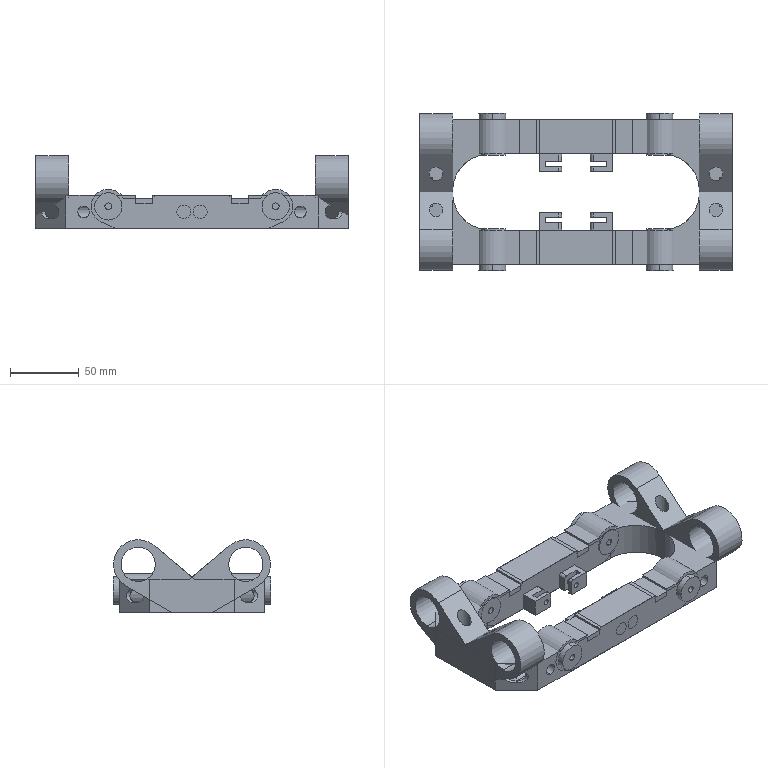NC program | Mastercam | posted with a generic post | part box 228 x 114.503 x 53 mm
Lines 1 to 1812 of 27132, first 1622 of 1812 lines:
%
:0001()
(MATERIAL - ALUMINUM MM - 2024)
(T24|100 FEM |H24)
(T16|16 FEM |H16|XY STOCK TO LEAVE - .15|Z STOCK TO LEAVE - 0.)
(T7|6 CHM |H7)
(T11|10 DR |H11)
(T23|50 FEM |H23|XY STOCK TO LEAVE - .3|Z STOCK TO LEAVE - 0.)
(T10|10 FEM |H10|XY STOCK TO LEAVE - .01|Z STOCK TO LEAVE - 0.)
(T9|10 DR |H9)
(T12|12 FEM |H12|XY STOCK TO LEAVE - .5|Z STOCK TO LEAVE - .2)
(T5|5 DR |H5)
(T6|6 FEM |H6|XY STOCK TO LEAVE - -.05|Z STOCK TO LEAVE - 0.)
(T13|10 BNOS |H13)
(T17|5 BM/BNOS |H17)
N100 G21
N102 G0 G17 G40 G80 G90 G94 G98
N104 G0 G28 G91 Z0.
N106 G0 G28 X0. Y0.
(100 FEM |TOOL - 24|DIA. OFF. - 24|LEN. - 24|TOOL DIA. - 100.)
N108 T24 M6
N110 G0 G54 G90 X-184. Y34.998 C0. B0. S4000 M3
N112 G43 H24 Z25.
N114 Z10.
N116 G1 Z0. F600.
N118 X134. F1200.
N120 G2 X168.998 Y0. J-34.998
N122 X134. Y-34.998 I-34.998
N124 G1 X-184.
N126 G0 Z25.
N128 M5
N130 G0 G28 G91 Z0.
N132 G28
N134 M01
N136 G0 G17 G40 G80 G90 G94 G98
N138 G0 G28 G91 Z0.
(16 FEM |TOOL - 16|DIA. OFF. - 16|LEN. - 16|TOOL DIA. - 16.)
N140 T16 M6
N142 G0 G54 G90 X-123.705 Y-71.319 C0. B0. S8250 M3
N144 G43 H16 Z50.
N146 Z3.
N148 G1 Z-53.3 F600.
N150 X-124.522 Y-69.286 F4000.
N152 X-125.029 Y-68.026
N154 G3 X-125.824 Y-66.824 I-3.34 J-1.343
N156 G1 X-126.147 Y-66.363
N158 X-126.473 Y-65.871
N160 X-126.833 Y-65.268
N162 X-127.184 Y-64.581
N164 X-127.476 Y-63.894
N166 X-127.702 Y-63.25
N168 X-127.876 Y-62.65
N170 X-128.009 Y-62.093
N172 X-128.112 Y-61.577
N174 X-128.191 Y-61.096
N176 X-128.298 Y-60.248
N178 X-128.365 Y-59.48
N180 X-128.407 Y-58.772
N182 G2 X-128.45 Y-57.477 I47.576 J2.234
N184 X-128.471 Y-55.217 I122.465 J2.26
N186 G1 Y-55.116
N188 G2 X-128.462 Y-51.17 I996.713 J-.393
N190 G1 X-128.46 Y-50.609
N192 X-128.25 Y5.613
N194 X-128.058 Y56.95
N196 X-128.05 Y57.685
N198 X-128.029 Y58.177
N200 X-127.985 Y58.725
N202 X-127.91 Y59.316
N204 X-127.797 Y59.933
N206 X-127.642 Y60.566
N208 X-127.44 Y61.204
N210 X-127.19 Y61.835
N212 X-126.891 Y62.451
N214 X-126.547 Y63.041
N216 X-126.165 Y63.599
N218 X-125.751 Y64.122
N220 X-125.311 Y64.608
N222 X-124.851 Y65.056
N224 X-124.376 Y65.466
N226 X-123.892 Y65.839
N228 X-123.404 Y66.177
N230 X-122.914 Y66.482
N232 X-122.426 Y66.755
N234 X-121.942 Y67.
N236 X-121.464 Y67.219
N238 X-120.994 Y67.415
N240 X-120.532 Y67.589
N242 X-120.08 Y67.744
N244 X-119.637 Y67.881
N246 X-119.204 Y68.004
N248 X-118.382 Y68.207
N250 X-117.593 Y68.369
N252 X-116.834 Y68.498
N254 X-116.102 Y68.602
N256 X-115.395 Y68.685
N258 X-114.709 Y68.752
N260 G2 X-113.389 Y68.851 I4.24 J-48.055
N262 X-111.506 Y68.939 I4.246 J-70.131
N264 X-108.513 Y69.008 I4.662 J-138.634
N266 X-103.882 Y69.041 I5.546 J-453.218
N268 G1 X-103.309 Y69.042
N270 X-98.736 Y69.048
N272 X-55.423 Y69.05
N274 X1.563
N276 X58.549
N278 X115.535
N280 X116.118
N282 X116.955 Y69.034
N284 X117.484 Y69.001
N286 X118.06 Y68.941
N288 X118.668 Y68.845
N290 X119.297 Y68.708
N292 X119.935 Y68.526
N294 X120.57 Y68.296
N296 X121.194 Y68.018
N298 X121.796 Y67.693
N300 X122.368 Y67.326
N302 X122.906 Y66.925
N304 X123.408 Y66.495
N306 X123.872 Y66.042
N308 X124.298 Y65.573
N310 X124.687 Y65.092
N312 X125.039 Y64.605
N314 X125.357 Y64.115
N316 X125.644 Y63.626
N318 X125.901 Y63.14
N320 X126.13 Y62.66
N322 X126.335 Y62.187
N324 X126.518 Y61.721
N326 X126.681 Y61.265
N328 X126.825 Y60.818
N330 X126.954 Y60.381
N332 X127.069 Y59.953
N334 X127.259 Y59.141
N336 X127.41 Y58.361
N338 X127.531 Y57.61
N340 X127.629 Y56.886
N342 X127.707 Y56.186
N344 X127.77 Y55.505
N346 G2 X127.896 Y53.56 I-52.944 J-4.404
N348 X127.979 Y51.111 I-97.529 J-4.546
N350 X128.027 Y47.588 I-234.327 J-4.98
N352 X128.047 Y41.847 I-980.786 J-6.151
N354 G1 Y41.276
N356 X128.05 Y28.162
N358 Y-28.824
N360 Y-56.747
N362 X128.048 Y-57.392
N364 X128.038 Y-57.841
N366 X128.01 Y-58.357
N368 X127.957 Y-58.923
N370 X127.87 Y-59.525
N372 X127.743 Y-60.151
N374 X127.572 Y-60.787
N376 X127.354 Y-61.424
N378 X127.086 Y-62.051
N380 X126.771 Y-62.659
N382 X126.414 Y-63.239
N384 X126.02 Y-63.785
N386 X125.596 Y-64.295
N388 X125.148 Y-64.768
N390 X124.682 Y-65.203
N392 X124.204 Y-65.6
N394 X123.718 Y-65.961
N396 X123.228 Y-66.287
N398 X122.739 Y-66.58
N400 X122.252 Y-66.844
N402 X121.77 Y-67.079
N404 X121.295 Y-67.29
N406 X120.828 Y-67.478
N408 X120.369 Y-67.645
N410 X119.92 Y-67.793
N412 X119.481 Y-67.926
N414 X119.051 Y-68.043
N416 X118.235 Y-68.238
N418 X117.451 Y-68.394
N420 X116.697 Y-68.519
N422 X115.97 Y-68.618
N424 X115.267 Y-68.698
N426 X114.584 Y-68.763
N428 G2 X112.634 Y-68.892 I-4.417 J51.948
N430 X110.181 Y-68.977 I-4.553 J95.562
N432 X106.656 Y-69.027 I-4.983 J229.371
N434 X100.914 Y-69.046 I-6.152 J959.501
N436 G1 X100.343 Y-69.047
N438 X87.229 Y-69.05
N440 X30.243
N442 X-26.743
N444 X-83.729
N446 X-116.249 Y-69.049
N448 X-116.668 Y-69.043
N450 X-117.162 Y-69.023
N452 X-117.818 Y-68.964
N454 X-118.488 Y-68.855
N456 X-119.15 Y-68.696
N458 X-119.798 Y-68.491
N460 X-120.427 Y-68.24
N462 X-121.033 Y-67.947
N464 X-121.615 Y-67.614
N466 X-122.164 Y-67.248
N468 X-122.684 Y-66.851
N470 X-123.168 Y-66.431
N472 X-123.62 Y-65.988
N474 X-124.037 Y-65.532
N476 X-124.42 Y-65.062
N478 X-124.77 Y-64.586
N480 X-125.089 Y-64.105
N482 X-125.377 Y-63.624
N484 X-125.638 Y-63.143
N486 X-125.872 Y-62.668
N488 X-126.083 Y-62.196
N490 X-126.271 Y-61.732
N492 X-126.44 Y-61.275
N494 X-126.591 Y-60.828
N496 X-126.725 Y-60.388
N498 X-126.845 Y-59.957
N500 X-127.044 Y-59.138
N502 X-127.203 Y-58.35
N504 X-127.33 Y-57.592
N506 X-127.431 Y-56.86
N508 X-127.512 Y-56.153
N510 X-127.577 Y-55.466
N512 G2 X-127.672 Y-54.145 I47.835 J4.073
N514 X-127.754 Y-52.26 I69.66 J3.993
N516 X-127.812 Y-49.266 I137.436 J4.152
N518 X-127.829 Y-45.396 I448.832 J3.87
N520 X-127.828 Y-44.634 I448.849
N522 G1 X-127.827 Y-44.061
N524 X-127.816 Y-39.488
N526 X-127.665 Y1.546
N528 X-127.466 Y54.557
N530 X-127.458 Y55.223
N532 X-127.426 Y56.064
N534 X-127.382 Y56.605
N536 X-127.307 Y57.19
N538 X-127.198 Y57.79
N540 X-127.055 Y58.393
N542 X-126.876 Y58.991
N544 X-126.664 Y59.579
N546 X-126.418 Y60.154
N548 X-126.142 Y60.711
N550 X-125.838 Y61.248
N552 X-125.508 Y61.762
N554 X-125.155 Y62.253
N556 X-124.781 Y62.719
N558 X-124.388 Y63.162
N560 X-123.985 Y63.574
N562 X-123.566 Y63.964
N564 X-123.142 Y64.325
N566 X-122.706 Y64.665
N568 X-122.27 Y64.977
N570 X-121.826 Y65.269
N572 X-121.385 Y65.537
N574 X-120.941 Y65.785
N576 X-120.502 Y66.013
N578 X-120.062 Y66.222
N580 X-119.628 Y66.414
N582 X-119.197 Y66.59
N584 X-118.772 Y66.751
N586 X-118.35 Y66.898
N588 X-117.542 Y67.151
N590 X-116.754 Y67.363
N592 X-115.987 Y67.54
N594 X-115.24 Y67.687
N596 X-114.514 Y67.811
N598 X-113.805 Y67.914
N600 X-113.114 Y68.
N602 X-112.438 Y68.072
N604 G2 X-110.487 Y68.225 I5.033 J-51.619
N606 X-108.015 Y68.337 I5.108 J-85.662
N608 X-104.46 Y68.409 I5.451 J-179.817
N610 X-99.269 Y68.441 I6.091 J-567.918
N612 G1 X-98.696 Y68.443
N614 X-92.985 Y68.449
N616 X-35.996 Y68.45
N618 X20.99
N620 X77.976
N622 X113.319
N624 X113.942 Y68.447
N626 X114.705 Y68.43
N628 X115.187 Y68.404
N630 X115.747 Y68.353
N632 X116.339 Y68.271
N634 X116.942 Y68.154
N636 X117.545 Y68.001
N638 X118.143 Y67.814
N640 X118.728 Y67.593
N642 X119.298 Y67.34
N644 X119.851 Y67.056
N646 X120.383 Y66.745
N648 X120.892 Y66.408
N650 X121.377 Y66.049
N652 X121.836 Y65.671
N654 X122.272 Y65.274
N656 X122.679 Y64.866
N658 X123.061 Y64.446
N660 X123.417 Y64.018
N662 X123.749 Y63.582
N664 X124.056 Y63.144
N666 X124.342 Y62.701
N668 X124.604 Y62.26
N670 X124.847 Y61.817
N672 X125.069 Y61.378
N674 X125.275 Y60.939
N676 X125.462 Y60.506
N678 X125.634 Y60.076
N680 X125.791 Y59.652
N682 X125.935 Y59.232
N684 X126.182 Y58.426
N686 X126.388 Y57.64
N688 X126.561 Y56.876
N690 X126.705 Y56.133
N692 X126.826 Y55.408
N694 X126.926 Y54.703
N696 X127.011 Y54.013
N698 X127.081 Y53.339
N700 G2 X127.23 Y51.393 I-52.557 J-5.016
N702 X127.339 Y48.925 I-87.362 J-5.097
N704 X127.41 Y45.373 I-183.675 J-5.444
N706 X127.442 Y40.183 I-580.792 J-6.088
N708 G1 X127.443 Y39.61
N710 X127.449 Y33.9
N712 X127.45 Y-23.089
N714 Y-54.443
N716 X127.445 Y-55.095
N718 X127.421 Y-55.903
N720 X127.386 Y-56.424
N722 X127.322 Y-57.002
N724 X127.224 Y-57.6
N726 X127.092 Y-58.205
N728 X126.925 Y-58.805
N730 X126.722 Y-59.398
N732 X126.487 Y-59.978
N734 X126.22 Y-60.541
N736 X125.925 Y-61.084
N738 X125.602 Y-61.605
N740 X125.256 Y-62.104
N742 X124.888 Y-62.579
N744 X124.5 Y-63.029
N746 X124.098 Y-63.453
N748 X123.685 Y-63.848
N750 X123.261 Y-64.219
N752 X122.83 Y-64.564
N754 X122.392 Y-64.886
N756 X121.952 Y-65.183
N758 X121.509 Y-65.459
N760 X121.067 Y-65.712
N762 X120.625 Y-65.946
N764 X120.186 Y-66.161
N766 X119.75 Y-66.358
N768 X119.318 Y-66.539
N770 X118.891 Y-66.704
N772 X118.468 Y-66.855
N774 X117.656 Y-67.115
N776 X116.865 Y-67.333
N778 X116.095 Y-67.515
N780 X115.345 Y-67.667
N782 X114.615 Y-67.793
N784 X113.904 Y-67.899
N786 X113.21 Y-67.988
N788 X112.532 Y-68.062
N790 G2 X110.575 Y-68.219 I-5.052 J50.585
N792 X108.099 Y-68.334 I-5.12 J83.809
N794 X104.541 Y-68.408 I-5.458 J175.663
N796 X99.348 Y-68.441 I-6.094 J554.097
N798 G1 X98.775 Y-68.442
N800 X93.634 Y-68.448
N802 X36.645 Y-68.45
N804 X-20.342
N806 X-77.328
N808 X-113.232
N810 X-113.862 Y-68.448
N812 X-114.281 Y-68.44
N814 X-114.789 Y-68.417
N816 X-115.345 Y-68.369
N818 X-115.925 Y-68.293
N820 X-116.517 Y-68.185
N822 X-117.112 Y-68.043
N824 X-117.703 Y-67.867
N826 X-118.284 Y-67.659
N828 X-118.854 Y-67.418
N830 X-119.407 Y-67.148
N832 X-119.941 Y-66.85
N834 X-120.455 Y-66.526
N836 X-120.945 Y-66.18
N838 X-121.412 Y-65.813
N840 X-121.855 Y-65.428
N842 X-122.275 Y-65.026
N844 X-122.665 Y-64.616
N846 X-123.034 Y-64.192
N848 X-123.375 Y-63.764
N850 X-123.695 Y-63.328
N852 X-123.991 Y-62.89
N854 X-124.265 Y-62.448
N856 X-124.518 Y-62.008
N858 X-124.752 Y-61.567
N860 X-124.966 Y-61.13
N862 X-125.163 Y-60.694
N864 X-125.344 Y-60.263
N866 X-125.51 Y-59.835
N868 X-125.661 Y-59.413
N870 X-125.922 Y-58.601
N872 X-126.14 Y-57.808
N874 X-126.323 Y-57.036
N876 X-126.475 Y-56.285
N878 X-126.602 Y-55.553
N880 X-126.708 Y-54.84
N882 X-126.796 Y-54.144
N884 X-126.87 Y-53.464
N886 G2 X-126.982 Y-52.144 I47.754 J4.723
N888 X-127.089 Y-50.246 I65.09 J4.62
N890 X-127.175 Y-47.222 I114.701 J4.772
N892 X-127.21 Y-43.137 I286.073 J4.496
N894 X-127.212 Y-41.018 I987.744 J2.119
N896 X-127.209 Y-38.545 I987.746
N898 G1 X-127.208 Y-37.974
N900 X-127.182 Y-29.987
N902 X-126.97 Y27.
N904 X-126.875 Y52.087
N906 X-126.87 Y52.701
N908 X-126.854 Y53.418
N910 X-126.836 Y53.838
N912 X-126.805 Y54.297
N914 X-126.758 Y54.784
N916 X-126.691 Y55.296
N918 X-126.602 Y55.823
N920 X-126.489 Y56.362
N922 X-126.35 Y56.903
N924 X-126.185 Y57.447
N926 X-125.994 Y57.987
N928 X-125.777 Y58.518
N930 X-125.536 Y59.039
N932 X-125.271 Y59.549
N934 X-124.984 Y60.044
N936 X-124.676 Y60.522
N938 X-124.349 Y60.983
N940 X-124.006 Y61.425
N942 X-123.647 Y61.848
N944 X-123.274 Y62.25
N946 X-122.887 Y62.636
N948 X-122.496 Y62.995
N950 X-122.092 Y63.339
N952 X-121.687 Y63.659
N954 X-121.272 Y63.963
N956 X-120.857 Y64.245
N958 X-120.437 Y64.511
N960 X-120.018 Y64.758
N962 X-119.597 Y64.99
N964 X-119.179 Y65.205
N966 X-118.76 Y65.405
N968 X-118.345 Y65.59
N970 X-117.932 Y65.763
N972 X-117.132 Y66.065
N974 X-116.346 Y66.324
N976 X-115.575 Y66.547
N978 X-114.819 Y66.738
N980 X-114.08 Y66.9
N982 X-113.356 Y67.039
N984 X-112.648 Y67.158
N986 X-111.954 Y67.259
N988 X-111.273 Y67.345
N990 G2 X-109.948 Y67.482 I5.4 J-45.953
N992 X-108.036 Y67.62 I5.334 J-60.429
N994 X-105.586 Y67.727 I5.426 J-95.971
N996 X-102.038 Y67.802 I5.759 J-188.499
N998 X-96.844 Y67.839 I6.362 J-539.267
N1000 G1 X-96.271 Y67.84
N1002 X-91.698 Y67.847
N1004 X-74.597 Y67.85
N1006 X-17.611
N1008 X39.375
N1010 X96.361
N1012 X111.199 Y67.849
N1014 X111.828 Y67.845
N1016 X112.578 Y67.827
N1018 X113.017 Y67.805
N1020 X113.488 Y67.768
N1022 X113.99 Y67.714
N1024 X114.51 Y67.639
N1026 X115.045 Y67.54
N1028 X115.586 Y67.417
N1030 X116.131 Y67.267
N1032 X116.674 Y67.091
N1034 X117.211 Y66.89
N1036 X117.739 Y66.663
N1038 X118.257 Y66.411
N1040 X118.762 Y66.136
N1042 X119.25 Y65.84
N1044 X119.721 Y65.524
N1046 X120.174 Y65.19
N1048 X120.608 Y64.84
N1050 X121.023 Y64.475
N1052 X121.419 Y64.096
N1054 X121.795 Y63.705
N1056 X122.146 Y63.31
N1058 X122.481 Y62.903
N1060 X122.793 Y62.494
N1062 X123.088 Y62.079
N1064 X123.363 Y61.662
N1066 X123.621 Y61.242
N1068 X123.862 Y60.822
N1070 X124.086 Y60.402
N1072 X124.294 Y59.983
N1074 X124.488 Y59.567
N1076 X124.668 Y59.152
N1078 X124.834 Y58.741
N1080 X125.126 Y57.944
N1082 X125.377 Y57.16
N1084 X125.593 Y56.392
N1086 X125.777 Y55.64
N1088 X125.934 Y54.904
N1090 X126.068 Y54.184
N1092 X126.182 Y53.479
N1094 X126.28 Y52.788
N1096 X126.363 Y52.11
N1098 G2 X126.495 Y50.79 I-47.152 J-5.367
N1100 X126.628 Y48.883 I-62.113 J-5.308
N1102 X126.732 Y46.439 I-98.875 J-5.406
N1104 X126.804 Y42.895 I-194.664 J-5.747
N1106 X126.839 Y37.703 I-558.221 J-6.356
N1108 G1 X126.841 Y37.13
N1110 X126.847 Y32.558
N1112 X126.85 Y14.318
N1114 Y-42.669
N1116 Y-51.792
N1118 Y-51.871
N1120 G2 X126.842 Y-53.047 I-84.373
N1122 G1 X126.815 Y-53.845
N1124 X126.784 Y-54.304
N1126 X126.737 Y-54.796
N1128 X126.671 Y-55.309
N1130 X126.581 Y-55.84
N1132 X126.467 Y-56.378
N1134 X126.327 Y-56.924
N1136 X126.162 Y-57.467
N1138 X125.97 Y-58.006
N1140 X125.752 Y-58.539
N1142 X125.51 Y-59.061
N1144 X125.244 Y-59.571
N1146 X124.956 Y-60.065
N1148 X124.648 Y-60.543
N1150 X124.321 Y-61.003
N1152 X123.976 Y-61.445
N1154 X123.616 Y-61.867
N1156 X123.24 Y-62.272
N1158 X122.855 Y-62.654
N1160 X122.462 Y-63.014
N1162 X122.059 Y-63.355
N1164 X121.652 Y-63.676
N1166 X121.239 Y-63.977
N1168 X120.822 Y-64.26
N1170 X120.404 Y-64.524
N1172 X119.983 Y-64.772
N1174 X119.564 Y-65.001
N1176 X119.143 Y-65.216
N1178 X118.727 Y-65.415
N1180 X118.31 Y-65.6
N1182 X117.899 Y-65.771
N1184 X117.099 Y-66.072
N1186 X116.313 Y-66.331
N1188 X115.542 Y-66.553
N1190 X114.787 Y-66.743
N1192 X114.047 Y-66.905
N1194 X113.324 Y-67.043
N1196 X112.616 Y-67.161
N1198 X111.922 Y-67.262
N1200 X111.242 Y-67.348
N1202 G2 X109.917 Y-67.484 I-5.395 J46.104
N1204 X108.005 Y-67.621 I-5.33 J60.648
N1206 X105.556 Y-67.728 I-5.421 J96.364
N1208 X102.009 Y-67.803 I-5.756 J189.366
N1210 X96.815 Y-67.839 I-6.361 J542.09
N1212 G1 X96.242 Y-67.84
N1214 X91.67 Y-67.847
N1216 X73.999 Y-67.85
N1218 X17.013
N1220 X-39.973
N1222 X-96.959
N1224 X-111.239 Y-67.849
N1226 X-111.938 Y-67.839
N1228 X-112.767 Y-67.804
N1230 X-113.238 Y-67.767
N1232 X-113.734 Y-67.713
N1234 X-114.25 Y-67.638
N1236 X-114.779 Y-67.54
N1238 X-115.315 Y-67.419
N1240 X-115.856 Y-67.272
N1242 X-116.395 Y-67.099
N1244 X-116.928 Y-66.901
N1246 X-117.456 Y-66.678
N1248 X-117.972 Y-66.43
N1250 X-118.475 Y-66.16
N1252 X-118.963 Y-65.868
N1254 X-119.434 Y-65.557
N1256 X-119.889 Y-65.227
N1258 X-120.325 Y-64.88
N1260 X-120.742 Y-64.519
N1262 X-121.141 Y-64.142
N1264 X-121.519 Y-63.756
N1266 X-121.874 Y-63.363
N1268 X-122.211 Y-62.96
N1270 X-122.528 Y-62.552
N1272 X-122.825 Y-62.14
N1274 X-123.105 Y-61.723
N1276 X-123.366 Y-61.306
N1278 X-123.611 Y-60.885
N1280 X-123.838 Y-60.467
N1282 X-124.05 Y-60.046
N1284 X-124.247 Y-59.631
N1286 X-124.431 Y-59.214
N1288 X-124.6 Y-58.803
N1290 X-124.898 Y-58.004
N1292 X-125.154 Y-57.218
N1294 X-125.373 Y-56.447
N1296 X-125.561 Y-55.692
N1298 X-125.721 Y-54.952
N1300 X-125.857 Y-54.229
N1302 X-125.974 Y-53.52
N1304 X-126.072 Y-52.826
N1306 X-126.157 Y-52.145
N1308 G2 X-126.289 Y-50.819 I45.956 J5.251
N1310 X-126.421 Y-48.906 I60.327 J5.13
N1312 X-126.52 Y-46.454 I95.553 J5.087
N1314 X-126.583 Y-42.906 I187.052 J5.073
N1316 X-126.601 Y-38.524 I532.903 J4.382
N1318 X-126.6 Y-37.71 I532.921
N1320 G1 Y-37.137
N1322 X-126.59 Y-32.565
N1324 X-126.528 Y-15.464
N1326 X-126.315 Y41.522
N1328 X-126.285 Y49.506
N1330 G2 X-126.275 Y50.715 I132.145 J-.472
N1332 G1 X-126.26 Y51.405
N1334 X-126.224 Y52.171
N1336 X-126.152 Y53.022
N1338 X-126.097 Y53.481
N1340 X-126.025 Y53.959
N1342 X-125.936 Y54.448
N1344 X-125.828 Y54.944
N1346 X-125.7 Y55.45
N1348 X-125.55 Y55.956
N1350 X-125.38 Y56.462
N1352 X-125.188 Y56.965
N1354 X-124.975 Y57.464
N1356 X-124.741 Y57.954
N1358 X-124.487 Y58.435
N1360 X-124.215 Y58.904
N1362 X-123.925 Y59.359
N1364 X-123.618 Y59.802
N1366 X-123.296 Y60.23
N1368 X-122.959 Y60.642
N1370 X-122.61 Y61.038
N1372 X-122.246 Y61.419
N1374 X-121.876 Y61.781
N1376 X-121.498 Y62.124
N1378 X-121.113 Y62.45
N1380 X-120.721 Y62.761
N1382 X-120.326 Y63.053
N1384 X-119.924 Y63.332
N1386 X-119.524 Y63.592
N1388 X-119.117 Y63.839
N1390 X-118.714 Y64.069
N1392 X-118.306 Y64.288
N1394 X-117.903 Y64.49
N1396 X-117.496 Y64.682
N1398 X-117.095 Y64.86
N1400 X-116.311 Y65.177
N1402 X-115.536 Y65.454
N1404 X-114.772 Y65.695
N1406 X-114.021 Y65.905
N1408 X-113.283 Y66.087
N1410 X-112.559 Y66.244
N1412 X-111.847 Y66.381
N1414 X-111.148 Y66.499
N1416 X-110.462 Y66.601
N1418 X-109.787 Y66.689
N1420 G2 X-107.823 Y66.888 I5.947 J-48.869
N1422 X-105.319 Y67.049 I5.949 J-73.321
N1424 X-102.308 Y67.154 I5.807 J-123.455
N1426 X-98.217 Y67.216 I6.125 J-267.548
N1428 X-91.9 Y67.244 I7.146 J-912.565
N1430 G1 X-91.328
N1432 X-83.342 Y67.249
N1434 X-26.354 Y67.25
N1436 X30.632
N1438 X87.618
N1440 X108.714 Y67.249
N1442 G2 X109.959 Y67.24 I-.008 J-87.599
N1444 G1 X110.677 Y67.221
N1446 X111.482 Y67.175
N1448 X111.921 Y67.137
N1450 X112.381 Y67.084
N1452 X112.857 Y67.017
N1454 X113.344 Y66.933
N1456 X113.843 Y66.829
N1458 X114.347 Y66.705
N1460 X114.853 Y66.56
N1462 X115.362 Y66.394
N1464 X115.868 Y66.206
N1466 X116.368 Y65.997
N1468 X116.86 Y65.768
N1470 X117.342 Y65.519
N1472 X117.815 Y65.249
N1474 X118.276 Y64.962
N1476 X118.722 Y64.658
N1478 X119.153 Y64.338
N1480 X119.568 Y64.004
N1482 X119.967 Y63.657
N1484 X120.349 Y63.299
N1486 X120.717 Y62.926
N1488 X121.062 Y62.552
N1490 X121.394 Y62.165
N1492 X121.705 Y61.777
N1494 X122.004 Y61.379
N1496 X122.283 Y60.981
N1498 X122.549 Y60.576
N1500 X122.797 Y60.173
N1502 X123.032 Y59.766
N1504 X123.251 Y59.361
N1506 X123.457 Y58.955
N1508 X123.65 Y58.551
N1510 X123.831 Y58.147
N1512 X124.151 Y57.363
N1514 X124.431 Y56.588
N1516 X124.676 Y55.824
N1518 X124.888 Y55.072
N1520 X125.072 Y54.333
N1522 X125.232 Y53.608
N1524 X125.37 Y52.895
N1526 X125.49 Y52.196
N1528 X125.593 Y51.508
N1530 X125.682 Y50.833
N1532 G2 X125.826 Y49.513 I-46.813 J-5.774
N1534 X125.977 Y47.6 I-60.178 J-5.7
N1536 X126.098 Y45.142 I-91.92 J-5.769
N1538 X126.187 Y41.582 I-170.898 J-6.068
N1540 X126.234 Y36.375 I-451.713 J-6.627
N1542 G1 X126.236 Y35.801
N1544 X126.245 Y31.795
N1546 X126.25 Y22.67
N1548 Y-34.317
N1550 X126.249 Y-49.715
N1552 G2 X126.24 Y-50.957 I-88.346 J.019
N1554 G1 X126.221 Y-51.679
N1556 X126.175 Y-52.481
N1558 X126.136 Y-52.923
N1560 X126.084 Y-53.382
N1562 X126.017 Y-53.856
N1564 X125.932 Y-54.346
N1566 X125.828 Y-54.844
N1568 X125.705 Y-55.347
N1570 X125.56 Y-55.856
N1572 X125.394 Y-56.364
N1574 X125.206 Y-56.868
N1576 X124.997 Y-57.368
N1578 X124.767 Y-57.861
N1580 X124.517 Y-58.345
N1582 X124.248 Y-58.817
N1584 X123.961 Y-59.277
N1586 X123.657 Y-59.722
N1588 X123.338 Y-60.153
N1590 X123.004 Y-60.568
N1592 X122.656 Y-60.967
N1594 X122.295 Y-61.352
N1596 X121.925 Y-61.718
N1598 X121.549 Y-62.064
N1600 X121.164 Y-62.395
N1602 X120.774 Y-62.708
N1604 X120.378 Y-63.004
N1606 X119.978 Y-63.285
N1608 X119.576 Y-63.549
N1610 X119.171 Y-63.798
N1612 X118.767 Y-64.031
N1614 X118.359 Y-64.252
N1616 X117.955 Y-64.457
N1618 X117.549 Y-64.651
N1620 X117.148 Y-64.83
N1622 X116.363 Y-65.151
N1624 X115.588 Y-65.431
N1626 X114.824 Y-65.676
N1628 X114.072 Y-65.888
N1630 X113.333 Y-66.072
N1632 X112.607 Y-66.232
N1634 X111.894 Y-66.37
N1636 X111.195 Y-66.49
N1638 X110.507 Y-66.593
N1640 X109.831 Y-66.682
N1642 G2 X108.511 Y-66.826 I-5.773 J46.822
N1644 X106.598 Y-66.977 I-5.699 J60.193
N1646 X104.141 Y-67.098 I-5.768 J91.948
N1648 X100.58 Y-67.187 I-6.069 J170.962
N1650 X95.373 Y-67.234 I-6.626 J451.892
N1652 G1 X94.799 Y-67.236
N1654 X90.794 Y-67.245
N1656 X81.668 Y-67.25
N1658 X24.681
N1660 X-32.305
N1662 X-89.291
N1664 X-108.683 Y-67.249
N1666 G2 X-109.974 Y-67.235 I.05 J62.315
N1668 G1 X-110.724 Y-67.206
N1670 X-111.556 Y-67.147
N1672 X-112.007 Y-67.099
N1674 X-112.476 Y-67.036
N1676 X-112.958 Y-66.957
N1678 X-113.449 Y-66.86
N1680 X-113.95 Y-66.743
N1682 X-114.455 Y-66.606
N1684 X-114.96 Y-66.449
N1686 X-115.464 Y-66.269
N1688 X-115.965 Y-66.069
N1690 X-116.459 Y-65.847
N1692 X-116.945 Y-65.606
N1694 X-117.419 Y-65.345
N1696 X-117.882 Y-65.066
N1698 X-118.333 Y-64.77
N1700 X-118.77 Y-64.457
N1702 X-119.191 Y-64.129
N1704 X-119.596 Y-63.788
N1706 X-119.985 Y-63.435
N1708 X-120.36 Y-63.068
N1710 X-120.713 Y-62.696
N1712 X-121.051 Y-62.314
N1714 X-121.37 Y-61.928
N1716 X-121.675 Y-61.533
N1718 X-121.96 Y-61.138
N1720 X-122.233 Y-60.734
N1722 X-122.487 Y-60.333
N1724 X-122.73 Y-59.925
N1726 X-122.955 Y-59.521
N1728 X-123.168 Y-59.113
N1730 X-123.366 Y-58.71
N1732 X-123.553 Y-58.304
N1734 X-123.883 Y-57.518
N1736 X-124.172 Y-56.739
N1738 X-124.424 Y-55.972
N1740 X-124.644 Y-55.216
N1742 X-124.834 Y-54.473
N1744 X-124.998 Y-53.743
N1746 X-125.141 Y-53.026
N1748 X-125.264 Y-52.323
N1750 X-125.37 Y-51.631
N1752 X-125.461 Y-50.952
N1754 G2 X-125.608 Y-49.625 I45.261 J5.674
N1756 X-125.759 Y-47.703 I57.98 J5.542
N1758 X-125.878 Y-45.237 I88.105 J5.486
N1760 X-125.96 Y-41.67 I162.826 J5.494
N1762 X-125.989 Y-37.032 I410.887 J4.902
N1764 X-125.99 Y-35.639 I976.491 J1.393
N1766 X-125.989 Y-34.737 I976.492
N1768 G1 Y-34.164
N1770 X-125.977 Y-29.023
N1772 X-125.896 Y-6.794
N1774 X-125.693 Y47.35
N1776 G2 X-125.673 Y49.179 I120.498 J-.39
N1778 G1 X-125.653 Y49.859
N1780 X-125.615 Y50.602
N1782 X-125.548 Y51.403
N1784 X-125.5 Y51.831
N1786 X-125.44 Y52.273
N1788 X-125.366 Y52.729
N1790 X-125.277 Y53.193
N1792 X-125.173 Y53.664
N1794 X-125.052 Y54.142
N1796 X-124.913 Y54.624
N1798 X-124.756 Y55.106
N1800 X-124.581 Y55.587
N1802 X-124.387 Y56.065
N1804 X-124.174 Y56.54
N1806 X-123.944 Y57.008
N1808 X-123.696 Y57.467
N1810 X-123.432 Y57.917
N1812 X-123.152 Y58.355
N1814 X-122.857 Y58.782
N1816 X-122.548 Y59.197
N1818 X-122.226 Y59.598
N1820 X-121.892 Y59.986
N1822 X-121.594 Y60.31
N1824 G3 X-121.484 Y60.479 I-.441 J.406
N1826 G2 X-114.934 Y65.348 I7.484 J-3.227
N1828 G3 X-113.341 Y65.574 I-12.858 J96.247
N1830 G2 X-110.932 Y65.902 I15.367 J-103.911
N1832 X-106.591 Y66.311 I9.422 J-76.87
N1834 X-102.958 Y66.49 I7.393 J-112.571
N1836 X-98.836 Y66.587 I6.862 J-204.835
N1838 X-93.064 Y66.634 I7.395 J-550.092
N1840 G1 X-92.491 Y66.636
N1842 X-88.487 Y66.645
N1844 X-79.362 Y66.649
N1846 X-22.375 Y66.65
N1848 X34.611
N1850 X91.597
N1852 X106.423 Y66.649
N1854 X106.459
N1856 G2 X108.262 Y66.635 J-109.067
N1858 G1 X108.96 Y66.614
N1860 X109.712 Y66.574
N1862 X110.524 Y66.504
N1864 X110.959 Y66.453
N1866 X111.406 Y66.39
N1868 X111.864 Y66.313
N1870 X112.334 Y66.22
N1872 X112.809 Y66.111
N1874 X113.289 Y65.985
N1876 X113.771 Y65.841
N1878 X114.255 Y65.678
N1880 X114.738 Y65.497
N1882 X115.107 Y65.345
N1884 G3 X115.244 Y65.306 I.228 J.554
N1886 G2 X120.759 Y61.807 I-1.244 J-8.054
N1888 G1 X121.208 Y61.14
N1890 X121.636 Y60.455
N1892 X122.04 Y59.75
N1894 X122.417 Y59.03
N1896 X122.766 Y58.301
N1898 X123.085 Y57.568
N1900 X123.374 Y56.833
N1902 X123.636 Y56.099
N1904 X123.871 Y55.37
N1906 X124.082 Y54.646
N1908 X124.27 Y53.929
N1910 X124.436 Y53.219
N1912 X124.584 Y52.518
N1914 X124.715 Y51.826
N1916 X124.83 Y51.143
N1918 X124.932 Y50.469
N1920 G2 X125.1 Y49.145 I-45.448 J-6.443
N1922 X125.282 Y47.218 I-56.248 J-6.304
N1924 X125.437 Y44.738 I-81.114 J-6.286
N1926 X125.543 Y41.737 I-130.44 J-6.121
N1928 X125.61 Y37.645 I-265.984 J-6.404
N1930 X125.642 Y31.324 I-834.44 J-7.374
N1932 G1 X125.643 Y30.752
N1934 X125.649 Y23.903
N1936 X125.65 Y-33.085
N1938 Y-47.339
N1940 Y-47.39
N1942 G2 X125.636 Y-49.166 I-119.967
N1944 G1 X125.618 Y-49.854
N1946 X125.581 Y-50.601
N1948 X125.517 Y-51.403
N1950 X125.469 Y-51.834
N1952 X125.409 Y-52.279
N1954 X125.336 Y-52.735
N1956 X125.248 Y-53.199
N1958 X125.144 Y-53.673
N1960 X125.022 Y-54.153
N1962 X124.883 Y-54.635
N1964 X124.726 Y-55.118
N1966 X124.55 Y-55.6
N1968 X124.356 Y-56.081
N1970 X124.143 Y-56.556
N1972 X123.912 Y-57.024
N1974 X123.664 Y-57.483
N1976 X123.4 Y-57.932
N1978 X123.119 Y-58.372
N1980 X122.823 Y-58.8
N1982 X122.513 Y-59.215
N1984 X122.19 Y-59.616
N1986 X121.856 Y-60.003
N1988 X121.61 Y-60.27
N1990 G3 X121.5 Y-60.441 I.442 J-.406
N1992 G2 X114.975 Y-65.343 I-7.5 J3.189
N1994 G3 X113.398 Y-65.565 I10.924 J-83.253
N1996 G2 X110.996 Y-65.893 I-15.996 J108.213
N1998 X106.654 Y-66.306 I-9.487 J76.831
N2000 X103.02 Y-66.488 I-7.414 J111.525
N2002 X98.895 Y-66.586 I-6.873 J202.287
N2004 X93.697 Y-66.632 I-7.008 J502.24
N2006 G1 X93.123 Y-66.634
N2008 X89.117 Y-66.644
N2010 X81.13 Y-66.649
N2012 X24.143 Y-66.65
N2014 X-32.844
N2016 X-89.83
N2018 X-106.369 Y-66.649
N2020 G2 X-107.587 Y-66.641 I.081 J108.567
N2022 G1 X-108.241 Y-66.629
N2024 X-108.956 Y-66.603
N2026 X-109.726 Y-66.554
N2028 X-110.553 Y-66.473
N2030 X-110.994 Y-66.415
N2032 X-111.446 Y-66.344
N2034 X-111.908 Y-66.258
N2036 X-112.381 Y-66.156
N2038 X-112.858 Y-66.038
N2040 X-113.337 Y-65.902
N2042 X-113.818 Y-65.749
N2044 X-114.301 Y-65.576
N2046 X-114.777 Y-65.387
N2048 G3 X-114.93 Y-65.349 I-.221 J-.558
N2050 G2 X-120.959 Y-61.494 I.93 J8.097
N2052 G1 X-121.347 Y-60.858
N2054 X-121.719 Y-60.192
N2056 X-122.076 Y-59.507
N2058 X-122.414 Y-58.806
N2060 X-122.729 Y-58.094
N2062 X-123.02 Y-57.376
N2064 X-123.286 Y-56.655
N2066 X-123.529 Y-55.934
N2068 X-123.748 Y-55.215
N2070 X-123.945 Y-54.5
N2072 X-124.122 Y-53.791
N2074 X-124.279 Y-53.088
N2076 X-124.419 Y-52.393
N2078 X-124.543 Y-51.706
N2080 X-124.652 Y-51.027
N2082 X-124.749 Y-50.357
N2084 G2 X-124.973 Y-48.391 I48.116 J6.498
N2086 X-125.162 Y-45.868 I67.448 J6.315
N2088 X-125.289 Y-42.83 I105.546 J5.925
N2090 X-125.362 Y-38.709 I209.206 J5.751
N2092 X-125.382 Y-33.777 I614.854 J4.932
N2094 X-125.381 Y-32.945 I614.874
N2096 G1 X-125.38 Y-32.372
N2098 X-125.371 Y-27.8
N2100 X-125.325 Y-14.687
N2102 X-125.112 Y42.299
N2104 X-125.098 Y45.734
N2106 G2 X-125.075 Y47.567 I112.781 J-.538
N2108 G1 X-125.054 Y48.231
N2110 X-125.02 Y48.941
N2112 X-124.964 Y49.696
N2114 X-124.879 Y50.498
N2116 X-124.756 Y51.337
N2118 X-124.676 Y51.778
N2120 X-124.581 Y52.229
N2122 X-124.473 Y52.686
N2124 X-124.35 Y53.146
N2126 X-124.212 Y53.609
N2128 X-124.057 Y54.073
N2130 X-123.885 Y54.538
N2132 X-123.7 Y54.994
N2134 X-123.511 Y55.422
N2136 X-123.149 Y56.172
N2138 X-122.811 Y56.818
N2140 X-122.161 Y58.004
N2142 G3 X-122.093 Y58.22 I-.527 J.287
N2144 G2 X-121.271 Y60.933 I8.093 J-.968
N2146 G3 X-120.883 Y62.559 I-3.212 J1.626
N2148 X-120.889 Y62.757 I-3.6
N2150 X-124.483 Y66.158 I-3.594 J-.198 F10000.
N2152 X-128.082 Y62.559 J-3.599
N2154 X-128.083 Y62.527 I3.599
N2156 G1 X-126.939 Y-64.414
N2158 G3 X-123.34 Y-67.981 I3.599 J.032
N2160 X-119.741 Y-64.382 J3.599
N2162 G1 X-119.748 Y-64.151
N2164 X-119.77 Y-63.921
N2166 G3 X-120.478 Y-62.197 I-3.571 J-.461 F4000.
N2168 G2 X-121.86 Y-59.406 I6.478 J4.945
N2170 G3 X-122.147 Y-58.435 I-53.177 J-15.167
N2172 G2 X-122.663 Y-56.699 I126.617 J38.571
N2174 X-123.007 Y-55.44 I50.789 J14.553
N2176 X-123.323 Y-54.143 I44.027 J11.435
N2178 G1 X-123.468 Y-53.488
N2180 X-123.602 Y-52.83
N2182 G2 X-123.841 Y-51.516 I44.605 J8.767
N2184 X-124.125 Y-49.563 I48.871 J8.114
N2186 X-124.389 Y-47.016 I60.467 J7.561
N2188 X-124.556 Y-44.538 I81.821 J6.761
N2190 X-124.692 Y-40.931 I128.315 J6.622
N2192 X-124.755 Y-36.832 I247.886 J5.892
N2194 X-124.773 Y-31.884 I674.114 J4.948
N2196 G1 Y-31.073
N2198 Y-30.501
N2200 X-124.764 Y-25.929
N2202 X-124.722 Y-13.955
N2204 X-124.509 Y43.035
N2206 G2 X-124.49 Y45.395 I213.759 J-.606
N2208 X-124.456 Y46.677 I59.968 J-.906
N2210 G1 X-124.425 Y47.363
N2212 X-124.377 Y48.084
N2214 X-124.306 Y48.846
N2216 X-124.206 Y49.643
N2218 X-124.069 Y50.47
N2220 X-123.895 Y51.301
N2222 X-123.688 Y52.115
N2224 X-123.455 Y52.895
N2226 X-123.207 Y53.635
N2228 X-122.956 Y54.317
N2230 G2 X-122.527 Y55.418 I171.263 J-66.046
N2232 G3 X-122.222 Y56.239 I-21.232 J8.345
N2234 G1 X-122.182 Y56.359
N2236 G3 X-122.15 Y56.551 I-.568 J.192
N2238 G1 Y57.121
N2240 Y57.252
N2242 G2 X-122.071 Y58.388 I8.15
N2244 G3 X-122.036 Y58.89 I-3.565 J.502
N2246 X-122.297 Y60.237 I-3.6
N2248 X-125.636 Y62.49 I-3.339 J-1.347 F10000.
N2250 X-129.236 Y58.89 J-3.6
N2252 X-129.235 Y58.869 I3.6
N2254 G1 X-128.545 Y-61.547
N2256 G3 X-124.945 Y-65.127 I3.6 J.02
N2258 X-121.386 Y-62.069 J3.6
N2260 X-121.345 Y-61.527 I-3.559 J.542 F4000.
N2262 X-121.592 Y-60.217 I-3.6
N2264 G2 X-122.136 Y-57.736 I7.592 J2.965
N2266 G3 X-122.259 Y-56.887 I-21.322 J-2.667
N2268 X-122.533 Y-55.341 I-70.644 J-11.705
N2270 G2 X-122.951 Y-53.001 I153.308 J28.63
N2272 X-123.486 Y-49.28 I71.891 J12.226
N2274 X-123.784 Y-46.174 I76.246 J8.888
N2276 X-123.994 Y-42.525 I104.408 J7.848
N2278 X-124.111 Y-38.377 I172.861 J6.947
N2280 X-124.161 Y-33.155 I376.486 J6.193
N2282 X-124.166 Y-29.894 I997.297 J3.261
N2284 X-124.165 Y-28.564 I997.302
N2286 G1 Y-27.992
N2288 X-124.151 Y-22.282
N2290 X-124.079 Y-2.332
N2292 X-123.914 Y41.555
N2294 G2 X-123.892 Y43.917 I202.323 J-.703
N2296 X-123.86 Y45.183 I67.301 J-1.099
N2298 G1 X-123.831 Y45.853
N2300 X-123.788 Y46.554
N2302 X-123.728 Y47.282
N2304 X-123.646 Y48.03
N2306 X-123.542 Y48.788
N2308 X-123.413 Y49.546
N2310 X-123.264 Y50.294
N2312 X-123.097 Y51.02
N2314 X-122.92 Y51.712
N2316 G2 X-122.561 Y52.98 I47.784 J-12.839
N2318 G3 X-122.258 Y54.008 I-103.838 J31.163
N2320 G1 X-122.172 Y54.32
N2322 G3 X-122.15 Y54.48 I-.578 J.16
N2324 G1 Y55.05
N2326 Y57.252
N2328 G3 X-122.633 Y59.052 I-3.6
N2330 X-125.75 Y60.851 I-3.117 J-1.8 F10000.
N2332 X-129.349 Y57.252 J-3.599
N2334 G1 Y57.247
N2336 X-129.192 Y-59.178
N2338 G3 X-125.592 Y-62.773 I3.6 J.005
N2340 X-122.222 Y-60.439 J3.6
N2342 X-121.992 Y-59.173 I-3.37 J1.266 F4000.
N2344 X-122.04 Y-58.585 I-3.6
N2346 G2 X-122.15 Y-57.252 I8.04 J1.333
N2348 G1 Y-56.682
N2350 Y-56.251
N2352 X-122.164 Y-55.873
N2354 G3 X-122.226 Y-55.001 I-23.058 J-1.19
N2356 X-122.383 Y-53.484 I-53.871 J-4.832
N2358 X-122.648 Y-51.23 I-517.451 J-59.755
N2360 G2 X-123.019 Y-47.643 I125.656 J14.799
N2362 X-123.339 Y-42.815 I115.484 J10.085
N2364 X-123.478 Y-38.665 I170.289 J7.76
N2366 X-123.547 Y-33.428 I325.586 J6.913
N2368 X-123.56 Y-28.393 I939.919 J5.035
N2370 X-123.559 Y-26.539 I939.932
N2372 G1 X-123.558 Y-25.967
N2374 X-123.544 Y-20.258
N2376 X-123.467 Y.831
N2378 X-123.322 Y39.588
N2380 G2 X-123.295 Y42.527 I251.108 J-.844
N2382 X-123.262 Y43.784 I72.817 J-1.26
N2384 X-123.197 Y45.116 I46.315 J-1.6
N2386 G1 X-123.146 Y45.808
N2388 X-123.081 Y46.512
N2390 X-122.999 Y47.222
N2392 X-122.902 Y47.931
N2394 X-122.79 Y48.634
N2396 X-122.666 Y49.322
N2398 X-122.533 Y49.99
N2400 G2 X-122.26 Y51.228 I62.214 J-13.029
N2402 G1 X-122.165 Y51.653
N2404 G3 X-122.15 Y51.785 I-.585 J.132
N2406 G1 Y52.354
N2408 Y55.204
N2410 G3 X-122.633 Y57.004 I-3.6
N2412 X-125.75 Y58.803 I-3.117 J-1.8 F10000.
N2414 X-129.35 Y55.204 J-3.599
N2416 G1 Y-57.105
N2418 G3 X-125.75 Y-60.705 I3.6
N2420 X-122.633 Y-58.905 J3.6
N2422 X-122.15 Y-57.105 I-3.117 J1.8 F4000.
N2424 G1 Y-56.251
N2426 Y-52.831
N2428 G3 X-122.171 Y-51.92 I-27.971 J-.176
N2430 X-122.251 Y-50.384 I-58.896 J-2.292
N2432 X-122.401 Y-48.154 I-361.876 J-23.294
N2434 G2 X-122.654 Y-44.055 I231.59 J16.334
N2436 X-122.866 Y-38.161 I197.881 J10.063
N2438 X-122.937 Y-32.932 I346.762 J7.382
N2440 X-122.955 Y-27.251 I914.949 J5.681
N2442 X-122.953 Y-25.467 I914.967
N2444 G1 Y-24.895
N2446 X-122.939 Y-19.186
N2448 X-122.876 Y-1.515
N2450 X-122.728 Y37.811
N2452 G2 X-122.705 Y40.729 I327.341 J-1.193
N2454 X-122.66 Y42.583 I90.427 J-1.259
N2456 X-122.598 Y43.882 I54.079 J-1.926
N2458 G1 X-122.553 Y44.548
N2460 X-122.497 Y45.221
N2462 X-122.43 Y45.897
N2464 X-122.352 Y46.572
N2466 X-122.263 Y47.242
N2468 X-122.157 Y47.957
N2470 G3 X-122.15 Y48.049 I-.593 J.092
N2472 G1 Y48.619
N2474 Y52.608
N2476 G3 X-122.633 Y54.408 I-3.6
N2478 X-125.75 Y56.207 I-3.117 J-1.8 F10000.
N2480 X-129.35 Y52.608 J-3.599
N2482 G1 Y-53.686
N2484 G3 X-125.75 Y-57.286 I3.6
N2486 X-122.633 Y-55.486 J3.6
N2488 X-122.15 Y-53.686 I-3.117 J1.8 F4000.
N2490 G1 Y-52.831
N2492 Y-44.775
N2494 G3 X-122.174 Y-42.616 I-126.282 J-.339
N2496 X-122.22 Y-40.355 I-935.96 J-17.695
N2498 G2 X-122.344 Y-29.982 I543.531 J11.694
N2500 X-122.349 Y-27.686 I988.76 J3.276
N2502 G1 X-122.35 Y-27.113
N2504 X-122.347 Y-23.109
N2506 X-122.331 Y-16.83
N2508 X-122.25 Y5.398
N2510 X-122.15 Y32.175
N2512 G3 X-122.149 Y32.748 I-304.977 J.573
N2514 X-122.15 Y33.317 I-304.978
N2516 G1 Y33.887
N2518 Y48.704
N2520 G3 X-122.633 Y50.504 I-3.6
N2522 X-125.75 Y52.303 I-3.117 J-1.8 F10000.
N2524 X-129.35 Y48.704 J-3.599
N2526 G1 Y-45.629
N2528 G3 X-125.75 Y-49.229 I3.6
N2530 X-122.633 Y-47.429 J3.6
N2532 X-122.15 Y-45.629 I-3.117 J1.8 F4000.
N2534 G1 Y-44.774
N2536 Y12.212
N2538 Y32.727
N2540 G3 X-122.439 Y34.139 I-3.6
N2542 G1 X-122.609 Y34.538
N2544 X-123.304 Y36.168 F10000.
N2546 G2 X-123.958 Y38.865 I7.752 J3.306
N2548 G1 X-125.43 Y59.185
N2550 G2 X-125.445 Y59.611 I5.884 J.426
N2552 X-119.546 Y65.51 I5.899
N2554 X-118.47 Y65.412 J-5.899
N2556 G1 X-117.645 Y65.259
N2558 X-117.218 Y65.179 F4000.
N2560 G3 X-116.562 Y65.119 I.656 J3.54
N2562 X-115.777 Y65.206 J3.6
N2564 G2 X-114. Y65.402 I1.777 J-7.954
N2566 G1 X-113.43
N2568 X-112.456
N2570 G3 X-111.522 Y65.427 I-.392 J31.763
N2572 X-109.942 Y65.508 I-3.374 J80.925
N2574 X-108.818 Y65.576 I-34.18 J578.183
N2576 G2 X-105.311 Y65.769 I15.088 J-242.104
N2578 X-100.011 Y65.945 I9.357 J-202.235
N2580 X-94.792 Y66.015 I7.829 J-386.667
N2582 X-89.628 Y66.039 I7.218 J-991.736
N2584 G1 X-89.056 Y66.041
N2586 X-83.347 Y66.048
N2588 X-58.838 Y66.05
N2590 X-1.852
N2592 X55.134
N2594 X104.728 Y66.049
N2596 G2 X106.565 Y66.031 I-.114 J-109.937
N2598 G1 X107.23 Y66.013
N2600 X107.943 Y65.98
N2602 X108.7 Y65.926
N2604 X109.504 Y65.843
N2606 X110.335 Y65.723
N2608 X111.094 Y65.584
N2610 X111.903 Y65.415
N2612 G3 X112.029 Y65.402 I.126 J.587
N2614 G1 X112.599
N2616 X114.
N2618 G2 X115.697 Y65.223 J-8.15
N2620 G3 X116.447 Y65.144 I.75 J3.521
N2622 X117.138 Y65.211 J3.6
N2624 G1 X117.564 Y65.295
N2626 X118.388 Y65.456 F10000.
N2628 G2 X118.504 Y65.467 I.116 J-.589
N2630 X118.813 Y65.381 J-.6
N2632 G1 X118.923 Y65.315
N2634 G2 X119.188 Y64.975 I-.309 J-.514
N2636 G1 X119.432 Y64.172
N2638 X119.558 Y63.757 F4000.
N2640 G3 X120.244 Y62.489 I3.445 J1.046
N2642 G2 X121.753 Y59.764 I-6.244 J-5.237
N2644 G3 X122.086 Y58.778 I72.615 J23.907
N2646 G2 X122.474 Y57.623 I-100.465 J-34.474
N2648 X122.869 Y56.375 I-49.189 J-16.22
N2650 G1 X123.058 Y55.729
N2652 X123.238 Y55.074
N2654 X123.409 Y54.414
N2656 X123.568 Y53.75
N2658 X123.716 Y53.085
N2660 X123.852 Y52.42
N2662 X123.977 Y51.757
N2664 G2 X124.194 Y50.44 I-44.93 J-8.082
N2666 X124.447 Y48.496 I-51.201 J-7.664
N2668 X124.679 Y45.972 I-66.213 J-7.346
N2670 X124.851 Y42.915 I-95.628 J-6.936
N2672 X124.958 Y39.352 I-167.269 J-6.806
N2674 X125.018 Y34.706 I-363.155 J-7.013
N2676 X125.039 Y30.114 I-965.181 J-6.718
N2678 G1 X125.041 Y29.542
N2680 X125.048 Y23.832
N2682 X125.05 Y-2.386
N2684 X125.049 Y-45.711
N2686 G2 X125.032 Y-47.545 I-111.888 J.113
N2688 G1 X125.014 Y-48.21
N2690 X124.981 Y-48.921
N2692 X124.928 Y-49.677
N2694 X124.845 Y-50.481
N2696 X124.725 Y-51.322
N2698 X124.645 Y-51.764
N2700 X124.552 Y-52.217
N2702 X124.444 Y-52.674
N2704 X124.322 Y-53.136
N2706 X124.184 Y-53.6
N2708 X124.03 Y-54.065
N2710 X123.859 Y-54.53
N2712 X123.675 Y-54.986
N2714 X123.488 Y-55.413
N2716 X123.13 Y-56.159
N2718 X122.796 Y-56.801
N2720 X122.164 Y-57.967
N2722 G3 X122.097 Y-58.183 I.529 J-.284
N2724 G2 X121.288 Y-60.9 I-8.097 J.931
N2726 G3 X120.907 Y-62.511 I3.22 J-1.611
N2728 X120.914 Y-62.725 I3.601
N2730 X124.508 Y-66.111 I3.594 J.214 F10000.
N2732 X128.108 Y-62.518 J3.6
N2734 G1 X128.337 Y62.018
N2736 Y62.024
N2738 G3 X124.737 Y65.624 I-3.6
N2740 X121.157 Y62.403 J-3.6
N2742 X121.137 Y62.024 I3.58 J-.379 F4000.
N2744 X121.448 Y60.562 I3.6
N2746 G2 X122.107 Y58.095 I-7.448 J-3.31
N2748 G3 X122.249 Y57.254 I20.759 J3.089
N2750 X122.561 Y55.704 I75.826 J14.436
N2752 G2 X123.032 Y53.347 I-122.299 J-25.68
N2754 X123.847 Y47.714 I-64.9 J-12.264
N2756 X124.101 Y44.625 I-82.148 J-8.306
N2758 X124.276 Y41.011 I-122.57 J-7.745
N2760 X124.376 Y36.895 I-215.729 J-7.294
N2762 X124.429 Y31.121 I-530.137 J-7.808
N2764 G1 X124.432 Y30.547
N2766 X124.443 Y26.542
N2768 X124.449 Y19.694
N2770 X124.45 Y-37.294
N2772 X124.449 Y-43.574
N2774 G2 X124.439 Y-45.357 I-186.133 J.166
N2776 X124.411 Y-46.639 I-60.138 J.677
N2778 G1 X124.382 Y-47.324
N2780 X124.337 Y-48.045
N2782 X124.269 Y-48.808
N2784 X124.172 Y-49.605
N2786 X124.039 Y-50.433
N2788 X123.867 Y-51.265
N2790 X123.663 Y-52.079
N2792 X123.434 Y-52.86
N2794 X123.189 Y-53.6
N2796 X122.941 Y-54.282
N2798 G2 X122.517 Y-55.384 I-178.755 J68.08
N2800 G3 X122.217 Y-56.205 I21.126 J-8.195
N2802 G1 X122.181 Y-56.312
N2804 G3 X122.15 Y-56.502 I.569 J-.19
N2806 G1 Y-57.072
N2808 Y-57.252
N2810 G2 X122.071 Y-58.388 I-8.15
N2812 G3 X122.036 Y-58.89 I3.565 J-.502
N2814 X122.297 Y-60.237 I3.6
N2816 X125.636 Y-62.49 I3.339 J1.347 F10000.
N2818 X129.236 Y-58.89 J3.6
N2820 G1 Y-58.885
N2822 X129.096 Y59.688
N2824 G3 X125.496 Y63.284 I-3.6 J-.004
N2826 X122.073 Y60.799 J-3.6
N2828 X121.896 Y59.684 I3.423 J-1.115 F4000.
N2830 X121.974 Y58.939 I3.6
N2832 G2 X122.15 Y57.252 I-7.974 J-1.687
N2834 G1 Y56.757
N2836 X122.167 Y56.397
N2838 G3 X122.238 Y55.55 I20.621 J1.307
N2840 X122.419 Y54.051 I49.075 J5.146
N2842 X122.645 Y52.381 I385.111 J51.278
N2844 G2 X123.02 Y49.412 I-139.962 J-19.197
N2846 X123.493 Y43.946 I-100.75 J-11.467
N2848 X123.681 Y39.768 I-144.242 J-8.582
N2850 X123.782 Y35.088 I-262.433 J-8.036
N2852 X123.832 Y28.753 I-644.927 J-8.255
N2854 G1 X123.834 Y28.18
N2856 X123.844 Y23.607
N2858 X123.849 Y14.481
N2860 Y-41.373
N2862 Y-41.453
N2864 G2 X123.838 Y-43.726 I-229.301
N2866 X123.813 Y-44.982 I-72.968 J.802
N2868 G1 X123.79 Y-45.645
N2870 X123.754 Y-46.335
N2872 X123.702 Y-47.053
N2874 X123.629 Y-47.796
N2876 X123.533 Y-48.555
N2878 X123.414 Y-49.316
N2880 X123.272 Y-50.069
N2882 X123.112 Y-50.802
N2884 X122.94 Y-51.505
N2886 X122.762 Y-52.17
N2888 G2 X122.42 Y-53.364 I-72.172 J20.078
N2890 G3 X122.172 Y-54.237 I34.974 J-10.391
N2892 X122.15 Y-54.397 I.578 J-.16
N2894 G1 Y-54.966
N2896 Y-57.252
N2898 G3 X122.633 Y-59.052 I3.6
N2900 X125.75 Y-60.851 I3.117 J1.8 F10000.
N2902 X129.349 Y-57.252 J3.599
N2904 G1 Y-57.251
N2906 X129.339 Y57.771
N2908 G3 X125.739 Y61.371 I-3.6
N2910 X122.545 Y59.431 J-3.6
N2912 X122.139 Y57.771 I3.194 J-1.66 F4000.
N2914 X122.142 Y57.612 I3.6
N2916 G2 X122.15 Y57.252 I-8.142 J-.36
N2918 G1 Y56.757
N2920 Y53.908
N2922 G3 X122.179 Y53.026 I24.027 J.337
N2924 X122.278 Y51.517 I50.264 J2.557
N2926 X122.465 Y49.301 I289.805 J23.26
N2928 G2 X122.744 Y45.785 I-213.024 J-18.708
N2930 X123.049 Y39.852 I-163.14 J-11.36
N2932 X123.172 Y34.593 I-267.713 J-8.904
N2934 X123.228 Y28.255 I-622.682 J-8.629
N2936 G1 X123.231 Y27.682
N2938 X123.242 Y23.678
N2940 X123.248 Y16.83
N2942 X123.25 Y-27.622
N2944 X123.248 Y-40.172
N2946 G2 X123.233 Y-42.539 I-191.4 J.094
N2948 X123.204 Y-43.798 I-71.437 J.998
N2950 X123.142 Y-45.13 I-45.798 J1.447
N2952 G1 X123.093 Y-45.822
N2954 X123.03 Y-46.526
N2956 X122.95 Y-47.236
N2958 X122.855 Y-47.945
N2960 X122.745 Y-48.647
N2962 X122.623 Y-49.334
N2964 G2 X122.357 Y-50.638 I-45.331 J8.552
N2966 G1 X122.227 Y-51.228
N2968 X122.164 Y-51.51
N2970 G3 X122.15 Y-51.64 I.586 J-.13
N2972 G1 Y-52.21
N2974 Y-55.059
N2976 G3 X122.633 Y-56.859 I3.6
N2978 X125.75 Y-58.658 I3.117 J1.8 F10000.
N2980 X129.35 Y-55.059 J3.599
N2982 G1 Y54.762
N2984 G3 X125.75 Y58.362 I-3.6
N2986 X122.633 Y56.562 J-3.6
N2988 X122.15 Y54.762 I3.117 J-1.8 F4000.
N2990 G1 Y53.908
N2992 Y48.209
N2994 G3 X122.182 Y46.668 I60.758 J.489
N2996 X122.288 Y43.886 I279.669 J9.262
N2998 G2 X122.472 Y38.671 I-373.202 J-15.752
N3000 X122.589 Y32.292 I-382.421 J-10.244
N3002 X122.636 Y24.829 I-925.123 J-9.454
N3004 G1 X122.637 Y24.257
N3006 X122.646 Y18.546
N3008 X122.65 Y4.295
N3010 X122.649 Y-37.882
N3012 Y-37.902
N3014 G2 X122.635 Y-40.805 I-305.615
N3016 X122.595 Y-42.665 I-86.691 J.95
N3018 X122.535 Y-43.969 I-52.846 J1.777
N3020 G1 X122.491 Y-44.636
N3022 X122.436 Y-45.31
N3024 X122.369 Y-45.986
N3026 X122.292 Y-46.661
N3028 X122.204 Y-47.329
N3030 X122.156 Y-47.665
N3032 G3 X122.15 Y-47.75 I.594 J-.085
N3034 G1 Y-48.32
N3036 Y-52.309
N3038 G3 X122.633 Y-54.109 I3.6
N3040 X125.75 Y-55.908 I3.117 J1.8 F10000.
N3042 X129.35 Y-52.309 J3.599
N3044 G1 Y49.064
N3046 G3 X125.75 Y52.664 I-3.6
N3048 X122.633 Y50.864 J-3.6
N3050 X122.15 Y49.064 I3.117 J-1.8 F4000.
N3052 G1 Y48.209
N3054 Y-8.777
N3056 Y-48.667
N3058 G3 X122.439 Y-50.079 I3.6
N3060 G1 X122.609 Y-50.478
N3062 X123.304 Y-52.109 F10000.
N3064 X125.323 Y-56.844
N3066 G2 X125.82 Y-59.279 I-5.711 J-2.435
N3068 X119.612 Y-65.487 I-6.208
N3070 X118.511 Y-65.389 J6.208
N3072 G1 X117.685 Y-65.24
N3074 X117.257 Y-65.163 F4000.
N3076 G3 X116.619 Y-65.106 I-.638 J-3.543
N3078 X115.817 Y-65.197 J-3.6
N3080 G2 X114. Y-65.402 I-1.817 J7.945
N3082 G1 X113.43
N3084 X112.44
N3086 G3 X111.505 Y-65.427 I.408 J-32.021
N3088 X109.923 Y-65.509 I3.42 J-81.654
N3090 X108.799 Y-65.576 I35.306 J-596.761
N3092 G2 X105.292 Y-65.769 I-15.041 J241.422
N3094 X99.993 Y-65.945 I-9.353 J202.377
N3096 X94.774 Y-66.015 I-7.828 J387.212
N3098 X89.61 Y-66.039 I-7.218 J993.409
N3100 G1 X89.038 Y-66.041
N3102 X83.328 Y-66.048
N3104 X58.82 Y-66.05
N3106 X1.834
N3108 X-55.152
N3110 X-104.17 Y-66.049
N3112 G2 X-105.974 Y-66.037 I.064 J147.81
N3114 X-107.307 Y-66. I.663 J46.852
N3116 G1 X-108.038 Y-65.959
N3118 X-108.816 Y-65.893
N3120 X-109.635 Y-65.794
N3122 X-110.436 Y-65.664
N3124 X-111.138 Y-65.529
N3126 X-111.693 Y-65.414
N3128 G3 X-111.815 Y-65.402 I-.122 J-.588
N3130 G1 X-112.385
N3132 X-114.
N3134 G2 X-115.136 Y-65.322 J8.15
N3136 G3 X-115.638 Y-65.287 I-.502 J-3.565
N3138 X-116.986 Y-65.549 J-3.6
N3140 X-119.238 Y-68.887 I1.348 J-3.338 F10000.
N3142 X-115.64 Y-72.487 I3.6
N3144 G1 X113.293 Y-72.602
N3146 X113.294
N3148 G3 X116.894 Y-69.002 J3.6
N3150 X115.094 Y-65.884 I-3.6
N3152 X113.294 Y-65.402 I-1.8 J-3.118 F4000.
N3154 G1 X112.44
N3156 X98.605
N3158 X95.205 Y-65.416
N3160 X90.634 Y-65.434
N3162 X85.493 Y-65.444
N3164 X75.798 Y-65.449
N3166 X18.811 Y-65.45
N3168 X-38.175
N3170 X-95.161
N3172 X-102.585 Y-65.448
N3174 G2 X-104.386 Y-65.435 I.221 J148.264
N3176 X-105.649 Y-65.402 I.845 J56.279
N3178 G1 X-106.218
N3180 X-112.487
N3182 G3 X-114.287 Y-65.884 J-3.6
N3184 X-116.087 Y-69.002 I1.8 J-3.118 F10000.
N3186 X-112.487 Y-72.602 I3.6
N3188 G1 X99.968
N3190 G3 X103.568 Y-69.002 J3.6
N3192 X101.768 Y-65.884 I-3.6
N3194 X99.968 Y-65.402 I-1.8 J-3.118 F4000.
N3196 G1 X99.113
N3198 X42.127
N3200 X-14.859
N3202 X-71.845
N3204 X-106.607
N3206 G3 X-108.019 Y-65.69 J-3.6
N3208 G1 X-108.418 Y-65.86
N3210 X-110.049 Y-66.556 F10000.
N3212 G2 X-114.48 Y-67.461 I-4.431 J10.392
N3214 X-125.777 Y-56.3 J11.297
N3216 G1 X-127.168 Y58.932
N3218 G2 X-127.169 Y59.028 I7.908 J.096
N3220 X-119.26 Y66.937 I7.909
N3222 X-116.158 Y66.302 J-7.909
N3224 G1 X-115.122 Y65.86
N3226 X-114.723 Y65.69 F4000.
N3228 G3 X-113.311 Y65.402 I1.412 J3.312
N3230 G1 X-112.456
N3232 X-98.608
N3234 X-94.637 Y65.419
N3236 X-90.065 Y65.436
N3238 X-84.925 Y65.445
N3240 X-74.091 Y65.45
N3242 X-17.104
N3244 X39.882
N3246 X96.868
N3248 X102.578 Y65.449
N3250 G2 X104.361 Y65.439 I-.166 J-185.11
N3252 X105.896 Y65.402 I-.656 J-58.961
N3254 G1 X106.466
N3256 X112.735
N3258 G3 X114.535 Y65.884 J3.6
N3260 X116.335 Y69.002 I-1.8 J3.118 F10000.
N3262 X112.735 Y72.602 I-3.6
N3264 G1 X-99.972
N3266 G3 X-103.572 Y69.002 J-3.6
N3268 X-101.772 Y65.884 I3.6
N3270 X-99.972 Y65.402 I1.8 J3.118 F4000.
N3272 G1 X-99.117
N3274 X-42.131
N3276 X14.855
N3278 X71.841
N3280 X106.603
N3282 G3 X108.015 Y65.69 J3.6
N3284 G1 X108.414 Y65.86
N3286 X110.044 Y66.556 F10000.
N3288 G0 Z50.
N3290 S5000 M3
N3292 X-115.6 Y68.552
N3294 Z46.7
N3296 Z-48.3
N3298 G1 Z-53.3 F600.
N3300 Y66.952 F1000.
N3302 G3 X-114. Y65.352 I1.6
N3304 G1 X114.
N3306 G2 X122.1 Y57.252 J-8.1
N3308 G1 Y-57.252